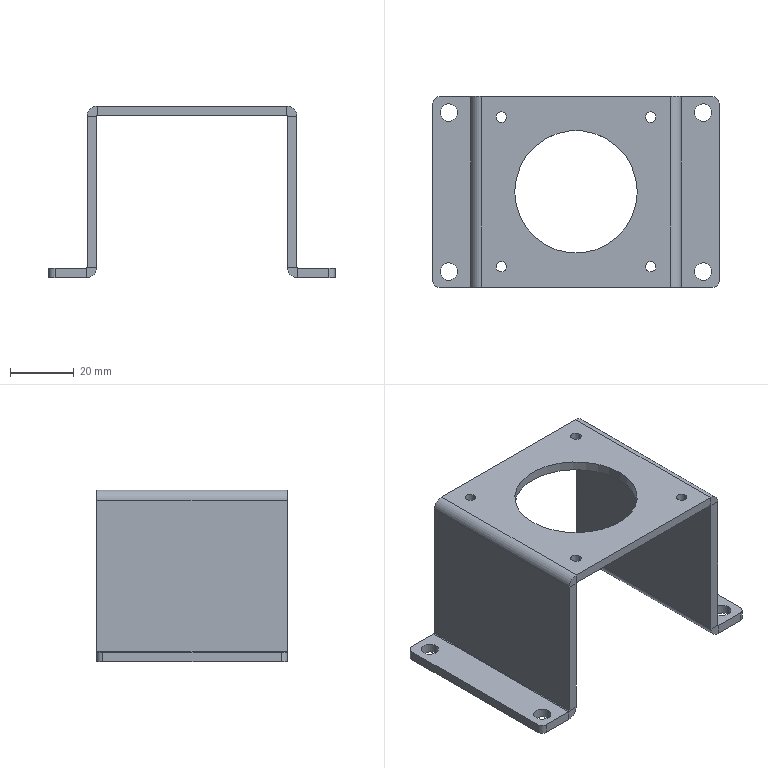Part | STEP file | 1 solid | 60 faces | box 90 x 60 x 54 mm | volume 30144 mm3 | cylinder 30 | plane 30 | commonest cylinder face diameters 3.3 x8 5.5 x8 0.4 x4 4 x4 6.4 x4 38.5 x2